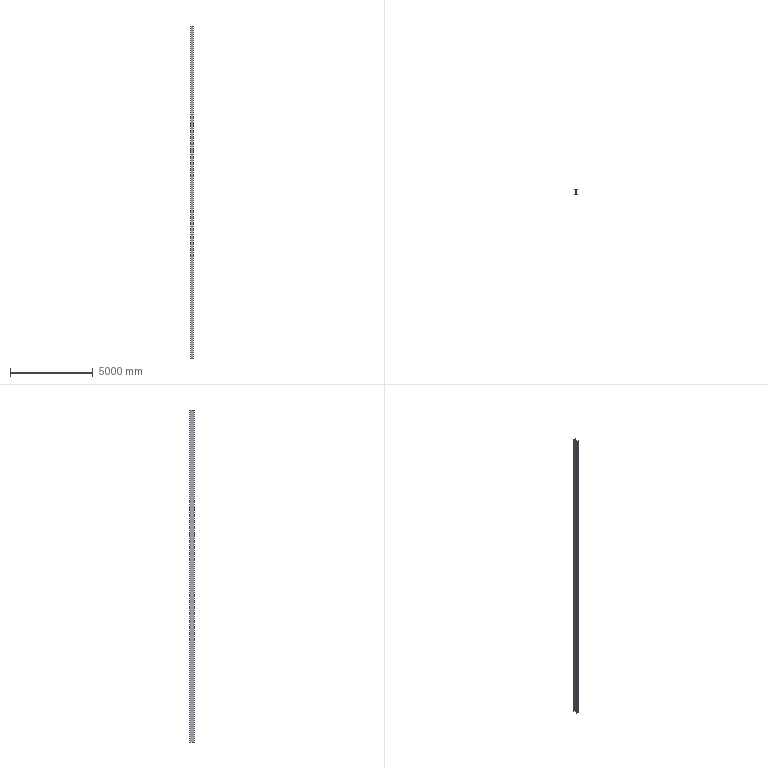Part | SolidWorks | features Extrusion 1 | 1 solid | 18 faces | box 150 x 300 x 20067 mm | volume 93874848 mm3 | plane 14 | cylinder 4 | commonest cylinder face diameters 26 x4
STEP:
#1=CARTESIAN_POINT('',(-75.,9.,0.));
#2=VERTEX_POINT('',#1);
#3=CARTESIAN_POINT('',(-75.,0.,0.));
#4=VERTEX_POINT('',#3);
#5=CARTESIAN_POINT('',(-75.,0.,0.));
#6=DIRECTION('',(0.,-1.,0.));
#7=VECTOR('',#6,1000.);
#8=LINE('',#5,#7);
#9=EDGE_CURVE('',#2,#4,#8,.T.);
#10=ORIENTED_EDGE('',*,*,#9,.T.);
#11=CARTESIAN_POINT('',(-75.,0.,20067.));
#12=VERTEX_POINT('',#11);
#13=CARTESIAN_POINT('',(-75.,0.,20067.));
#14=DIRECTION('',(0.,0.,-1.));
#15=VECTOR('',#14,1000.);
#16=LINE('',#13,#15);
#17=EDGE_CURVE('',#12,#4,#16,.T.);
#18=ORIENTED_EDGE('',*,*,#17,.F.);
#19=CARTESIAN_POINT('',(-75.,9.,20067.));
#20=VERTEX_POINT('',#19);
#21=CARTESIAN_POINT('',(-75.,0.,20067.));
#22=DIRECTION('',(0.,-1.,0.));
#23=VECTOR('',#22,1000.);
#24=LINE('',#21,#23);
#25=EDGE_CURVE('',#20,#12,#24,.T.);
#26=ORIENTED_EDGE('',*,*,#25,.F.);
#27=CARTESIAN_POINT('',(-75.,9.,20067.));
#28=DIRECTION('',(0.,0.,-1.));
#29=VECTOR('',#28,1000.);
#30=LINE('',#27,#29);
#31=EDGE_CURVE('',#20,#2,#30,.T.);
#32=ORIENTED_EDGE('',*,*,#31,.T.);
#33=EDGE_LOOP('',(#10,#18,#26,#32));
#34=FACE_OUTER_BOUND('',#33,.T.);
#35=CARTESIAN_POINT('',(-75.,0.,20067.));
#36=DIRECTION('',(1.,0.,0.));
#37=DIRECTION('',(0.,0.,-1.));
#38=AXIS2_PLACEMENT_3D('',#35,#36,#37);
#39=PLANE('',#38);
#40=ADVANCED_FACE('',(#34),#39,.F.);
#41=CARTESIAN_POINT('',(75.,0.,0.));
#42=VERTEX_POINT('',#41);
#43=CARTESIAN_POINT('',(75.,0.,0.));
#44=DIRECTION('',(1.,0.,0.));
#45=VECTOR('',#44,1000.);
#46=LINE('',#43,#45);
#47=EDGE_CURVE('',#4,#42,#46,.T.);
#48=ORIENTED_EDGE('',*,*,#47,.T.);
#49=CARTESIAN_POINT('',(75.,0.,20067.));
#50=VERTEX_POINT('',#49);
#51=CARTESIAN_POINT('',(75.,0.,20067.));
#52=DIRECTION('',(0.,0.,-1.));
#53=VECTOR('',#52,1000.);
#54=LINE('',#51,#53);
#55=EDGE_CURVE('',#50,#42,#54,.T.);
#56=ORIENTED_EDGE('',*,*,#55,.F.);
#57=CARTESIAN_POINT('',(75.,0.,20067.));
#58=DIRECTION('',(1.,0.,0.));
#59=VECTOR('',#58,1000.);
#60=LINE('',#57,#59);
#61=EDGE_CURVE('',#12,#50,#60,.T.);
#62=ORIENTED_EDGE('',*,*,#61,.F.);
#63=ORIENTED_EDGE('',*,*,#17,.T.);
#64=EDGE_LOOP('',(#48,#56,#62,#63));
#65=FACE_OUTER_BOUND('',#64,.T.);
#66=CARTESIAN_POINT('',(75.,0.,20067.));
#67=DIRECTION('',(0.,1.,0.));
#68=DIRECTION('',(-1.,0.,0.));
#69=AXIS2_PLACEMENT_3D('',#66,#67,#68);
#70=PLANE('',#69);
#71=ADVANCED_FACE('',(#65),#70,.F.);
#72=CARTESIAN_POINT('',(75.,9.,0.));
#73=VERTEX_POINT('',#72);
#74=CARTESIAN_POINT('',(75.,0.,0.));
#75=DIRECTION('',(0.,1.,0.));
#76=VECTOR('',#75,1000.);
#77=LINE('',#74,#76);
#78=EDGE_CURVE('',#42,#73,#77,.T.);
#79=ORIENTED_EDGE('',*,*,#78,.T.);
#80=CARTESIAN_POINT('',(75.,9.,20067.));
#81=VERTEX_POINT('',#80);
#82=CARTESIAN_POINT('',(75.,9.,20067.));
#83=DIRECTION('',(0.,0.,-1.));
#84=VECTOR('',#83,1000.);
#85=LINE('',#82,#84);
#86=EDGE_CURVE('',#81,#73,#85,.T.);
#87=ORIENTED_EDGE('',*,*,#86,.F.);
#88=CARTESIAN_POINT('',(75.,0.,20067.));
#89=DIRECTION('',(0.,1.,0.));
#90=VECTOR('',#89,1000.);
#91=LINE('',#88,#90);
#92=EDGE_CURVE('',#50,#81,#91,.T.);
#93=ORIENTED_EDGE('',*,*,#92,.F.);
#94=ORIENTED_EDGE('',*,*,#55,.T.);
#95=EDGE_LOOP('',(#79,#87,#93,#94));
#96=FACE_OUTER_BOUND('',#95,.T.);
#97=CARTESIAN_POINT('',(75.,0.,20067.));
#98=DIRECTION('',(-1.,0.,0.));
#99=DIRECTION('',(0.,0.,1.));
#100=AXIS2_PLACEMENT_3D('',#97,#98,#99);
#101=PLANE('',#100);
#102=ADVANCED_FACE('',(#96),#101,.F.);
#103=CARTESIAN_POINT('',(16.25,9.,0.));
#104=VERTEX_POINT('',#103);
#105=CARTESIAN_POINT('',(75.,9.,0.));
#106=DIRECTION('',(-1.,0.,0.));
#107=VECTOR('',#106,1000.);
#108=LINE('',#105,#107);
#109=EDGE_CURVE('',#73,#104,#108,.T.);
#110=ORIENTED_EDGE('',*,*,#109,.T.);
#111=CARTESIAN_POINT('',(16.25,9.,20067.));
#112=VERTEX_POINT('',#111);
#113=CARTESIAN_POINT('',(16.25,9.,20067.));
#114=DIRECTION('',(0.,0.,-1.));
#115=VECTOR('',#114,1000.);
#116=LINE('',#113,#115);
#117=EDGE_CURVE('',#112,#104,#116,.T.);
#118=ORIENTED_EDGE('',*,*,#117,.F.);
#119=CARTESIAN_POINT('',(75.,9.,20067.));
#120=DIRECTION('',(-1.,0.,0.));
#121=VECTOR('',#120,1000.);
#122=LINE('',#119,#121);
#123=EDGE_CURVE('',#81,#112,#122,.T.);
#124=ORIENTED_EDGE('',*,*,#123,.F.);
#125=ORIENTED_EDGE('',*,*,#86,.T.);
#126=EDGE_LOOP('',(#110,#118,#124,#125));
#127=FACE_OUTER_BOUND('',#126,.T.);
#128=CARTESIAN_POINT('',(75.,9.,20067.));
#129=DIRECTION('',(0.,-1.,0.));
#130=DIRECTION('',(1.,0.,0.));
#131=AXIS2_PLACEMENT_3D('',#128,#129,#130);
#132=PLANE('',#131);
#133=ADVANCED_FACE('',(#127),#132,.F.);
#134=CARTESIAN_POINT('',(3.25,22.,0.));
#135=VERTEX_POINT('',#134);
#136=CARTESIAN_POINT('',(16.25,22.,0.));
#137=DIRECTION('',(0.,0.,-1.));
#138=DIRECTION('',(-1.,0.,0.));
#139=AXIS2_PLACEMENT_3D('',#136,#137,#138);
#140=CIRCLE('',#139,13.);
#141=EDGE_CURVE('',#104,#135,#140,.T.);
#142=ORIENTED_EDGE('',*,*,#141,.T.);
#143=CARTESIAN_POINT('',(3.25,22.,20067.));
#144=VERTEX_POINT('',#143);
#145=CARTESIAN_POINT('',(3.25,22.,20067.));
#146=DIRECTION('',(0.,0.,-1.));
#147=VECTOR('',#146,1000.);
#148=LINE('',#145,#147);
#149=EDGE_CURVE('',#144,#135,#148,.T.);
#150=ORIENTED_EDGE('',*,*,#149,.F.);
#151=CARTESIAN_POINT('',(16.25,22.,20067.));
#152=DIRECTION('',(0.,0.,-1.));
#153=DIRECTION('',(-1.,0.,0.));
#154=AXIS2_PLACEMENT_3D('',#151,#152,#153);
#155=CIRCLE('',#154,13.);
#156=EDGE_CURVE('',#112,#144,#155,.T.);
#157=ORIENTED_EDGE('',*,*,#156,.F.);
#158=ORIENTED_EDGE('',*,*,#117,.T.);
#159=EDGE_LOOP('',(#142,#150,#157,#158));
#160=FACE_OUTER_BOUND('',#159,.T.);
#161=CARTESIAN_POINT('',(16.25,22.,20067.));
#162=DIRECTION('',(0.,0.,-1.));
#163=DIRECTION('',(-1.,0.,0.));
#164=AXIS2_PLACEMENT_3D('',#161,#162,#163);
#165=CYLINDRICAL_SURFACE('',#164,13.);
#166=ADVANCED_FACE('',(#160),#165,.F.);
#167=CARTESIAN_POINT('',(3.25,278.,0.));
#168=VERTEX_POINT('',#167);
#169=CARTESIAN_POINT('',(3.25,22.,0.));
#170=DIRECTION('',(0.,1.,0.));
#171=VECTOR('',#170,1000.);
#172=LINE('',#169,#171);
#173=EDGE_CURVE('',#135,#168,#172,.T.);
#174=ORIENTED_EDGE('',*,*,#173,.T.);
#175=CARTESIAN_POINT('',(3.25,278.,20067.));
#176=VERTEX_POINT('',#175);
#177=CARTESIAN_POINT('',(3.25,278.,20067.));
#178=DIRECTION('',(0.,0.,-1.));
#179=VECTOR('',#178,1000.);
#180=LINE('',#177,#179);
#181=EDGE_CURVE('',#176,#168,#180,.T.);
#182=ORIENTED_EDGE('',*,*,#181,.F.);
#183=CARTESIAN_POINT('',(3.25,22.,20067.));
#184=DIRECTION('',(0.,1.,0.));
#185=VECTOR('',#184,1000.);
#186=LINE('',#183,#185);
#187=EDGE_CURVE('',#144,#176,#186,.T.);
#188=ORIENTED_EDGE('',*,*,#187,.F.);
#189=ORIENTED_EDGE('',*,*,#149,.T.);
#190=EDGE_LOOP('',(#174,#182,#188,#189));
#191=FACE_OUTER_BOUND('',#190,.T.);
#192=CARTESIAN_POINT('',(3.25,22.,20067.));
#193=DIRECTION('',(-1.,0.,0.));
#194=DIRECTION('',(0.,0.,1.));
#195=AXIS2_PLACEMENT_3D('',#192,#193,#194);
#196=PLANE('',#195);
#197=ADVANCED_FACE('',(#191),#196,.F.);
#198=CARTESIAN_POINT('',(16.25,291.,0.));
#199=VERTEX_POINT('',#198);
#200=CARTESIAN_POINT('',(16.25,278.,0.));
#201=DIRECTION('',(0.,0.,-1.));
#202=DIRECTION('',(-1.,0.,0.));
#203=AXIS2_PLACEMENT_3D('',#200,#201,#202);
#204=CIRCLE('',#203,13.);
#205=EDGE_CURVE('',#168,#199,#204,.T.);
#206=ORIENTED_EDGE('',*,*,#205,.T.);
#207=CARTESIAN_POINT('',(16.25,291.,20067.));
#208=VERTEX_POINT('',#207);
#209=CARTESIAN_POINT('',(16.25,291.,20067.));
#210=DIRECTION('',(0.,0.,-1.));
#211=VECTOR('',#210,1000.);
#212=LINE('',#209,#211);
#213=EDGE_CURVE('',#208,#199,#212,.T.);
#214=ORIENTED_EDGE('',*,*,#213,.F.);
#215=CARTESIAN_POINT('',(16.25,278.,20067.));
#216=DIRECTION('',(0.,0.,-1.));
#217=DIRECTION('',(-1.,0.,0.));
#218=AXIS2_PLACEMENT_3D('',#215,#216,#217);
#219=CIRCLE('',#218,13.);
#220=EDGE_CURVE('',#176,#208,#219,.T.);
#221=ORIENTED_EDGE('',*,*,#220,.F.);
#222=ORIENTED_EDGE('',*,*,#181,.T.);
#223=EDGE_LOOP('',(#206,#214,#221,#222));
#224=FACE_OUTER_BOUND('',#223,.T.);
#225=CARTESIAN_POINT('',(16.25,278.,20067.));
#226=DIRECTION('',(0.,0.,-1.));
#227=DIRECTION('',(-1.,0.,0.));
#228=AXIS2_PLACEMENT_3D('',#225,#226,#227);
#229=CYLINDRICAL_SURFACE('',#228,13.);
#230=ADVANCED_FACE('',(#224),#229,.F.);
#231=CARTESIAN_POINT('',(75.,291.,0.));
#232=VERTEX_POINT('',#231);
#233=CARTESIAN_POINT('',(16.25,291.,0.));
#234=DIRECTION('',(1.,0.,0.));
#235=VECTOR('',#234,1000.);
#236=LINE('',#233,#235);
#237=EDGE_CURVE('',#199,#232,#236,.T.);
#238=ORIENTED_EDGE('',*,*,#237,.T.);
#239=CARTESIAN_POINT('',(75.,291.,20067.));
#240=VERTEX_POINT('',#239);
#241=CARTESIAN_POINT('',(75.,291.,20067.));
#242=DIRECTION('',(0.,0.,-1.));
#243=VECTOR('',#242,1000.);
#244=LINE('',#241,#243);
#245=EDGE_CURVE('',#240,#232,#244,.T.);
#246=ORIENTED_EDGE('',*,*,#245,.F.);
#247=CARTESIAN_POINT('',(16.25,291.,20067.));
#248=DIRECTION('',(1.,0.,0.));
#249=VECTOR('',#248,1000.);
#250=LINE('',#247,#249);
#251=EDGE_CURVE('',#208,#240,#250,.T.);
#252=ORIENTED_EDGE('',*,*,#251,.F.);
#253=ORIENTED_EDGE('',*,*,#213,.T.);
#254=EDGE_LOOP('',(#238,#246,#252,#253));
#255=FACE_OUTER_BOUND('',#254,.T.);
#256=CARTESIAN_POINT('',(16.25,291.,20067.));
#257=DIRECTION('',(0.,1.,0.));
#258=DIRECTION('',(-1.,0.,0.));
#259=AXIS2_PLACEMENT_3D('',#256,#257,#258);
#260=PLANE('',#259);
#261=ADVANCED_FACE('',(#255),#260,.F.);
#262=CARTESIAN_POINT('',(75.,300.,0.));
#263=VERTEX_POINT('',#262);
#264=CARTESIAN_POINT('',(75.,291.,0.));
#265=DIRECTION('',(0.,1.,0.));
#266=VECTOR('',#265,1000.);
#267=LINE('',#264,#266);
#268=EDGE_CURVE('',#232,#263,#267,.T.);
#269=ORIENTED_EDGE('',*,*,#268,.T.);
#270=CARTESIAN_POINT('',(75.,300.,20067.));
#271=VERTEX_POINT('',#270);
#272=CARTESIAN_POINT('',(75.,300.,20067.));
#273=DIRECTION('',(0.,0.,-1.));
#274=VECTOR('',#273,1000.);
#275=LINE('',#272,#274);
#276=EDGE_CURVE('',#271,#263,#275,.T.);
#277=ORIENTED_EDGE('',*,*,#276,.F.);
#278=CARTESIAN_POINT('',(75.,291.,20067.));
#279=DIRECTION('',(0.,1.,0.));
#280=VECTOR('',#279,1000.);
#281=LINE('',#278,#280);
#282=EDGE_CURVE('',#240,#271,#281,.T.);
#283=ORIENTED_EDGE('',*,*,#282,.F.);
#284=ORIENTED_EDGE('',*,*,#245,.T.);
#285=EDGE_LOOP('',(#269,#277,#283,#284));
#286=FACE_OUTER_BOUND('',#285,.T.);
#287=CARTESIAN_POINT('',(75.,291.,20067.));
#288=DIRECTION('',(-1.,0.,0.));
#289=DIRECTION('',(0.,-1.,0.));
#290=AXIS2_PLACEMENT_3D('',#287,#288,#289);
#291=PLANE('',#290);
#292=ADVANCED_FACE('',(#286),#291,.F.);
#293=CARTESIAN_POINT('',(-75.,300.,0.));
#294=VERTEX_POINT('',#293);
#295=CARTESIAN_POINT('',(-75.,300.,0.));
#296=DIRECTION('',(-1.,0.,0.));
#297=VECTOR('',#296,1000.);
#298=LINE('',#295,#297);
#299=EDGE_CURVE('',#263,#294,#298,.T.);
#300=ORIENTED_EDGE('',*,*,#299,.T.);
#301=CARTESIAN_POINT('',(-75.,300.,20067.));
#302=VERTEX_POINT('',#301);
#303=CARTESIAN_POINT('',(-75.,300.,20067.));
#304=DIRECTION('',(0.,0.,-1.));
#305=VECTOR('',#304,1000.);
#306=LINE('',#303,#305);
#307=EDGE_CURVE('',#302,#294,#306,.T.);
#308=ORIENTED_EDGE('',*,*,#307,.F.);
#309=CARTESIAN_POINT('',(-75.,300.,20067.));
#310=DIRECTION('',(-1.,0.,0.));
#311=VECTOR('',#310,1000.);
#312=LINE('',#309,#311);
#313=EDGE_CURVE('',#271,#302,#312,.T.);
#314=ORIENTED_EDGE('',*,*,#313,.F.);
#315=ORIENTED_EDGE('',*,*,#276,.T.);
#316=EDGE_LOOP('',(#300,#308,#314,#315));
#317=FACE_OUTER_BOUND('',#316,.T.);
#318=CARTESIAN_POINT('',(-75.,300.,20067.));
#319=DIRECTION('',(0.,-1.,0.));
#320=DIRECTION('',(0.,0.,-1.));
#321=AXIS2_PLACEMENT_3D('',#318,#319,#320);
#322=PLANE('',#321);
#323=ADVANCED_FACE('',(#317),#322,.F.);
#324=CARTESIAN_POINT('',(-75.,291.,0.));
#325=VERTEX_POINT('',#324);
#326=CARTESIAN_POINT('',(-75.,291.,0.));
#327=DIRECTION('',(0.,-1.,0.));
#328=VECTOR('',#327,1000.);
#329=LINE('',#326,#328);
#330=EDGE_CURVE('',#294,#325,#329,.T.);
#331=ORIENTED_EDGE('',*,*,#330,.T.);
#332=CARTESIAN_POINT('',(-75.,291.,20067.));
#333=VERTEX_POINT('',#332);
#334=CARTESIAN_POINT('',(-75.,291.,20067.));
#335=DIRECTION('',(0.,0.,-1.));
#336=VECTOR('',#335,1000.);
#337=LINE('',#334,#336);
#338=EDGE_CURVE('',#333,#325,#337,.T.);
#339=ORIENTED_EDGE('',*,*,#338,.F.);
#340=CARTESIAN_POINT('',(-75.,291.,20067.));
#341=DIRECTION('',(0.,-1.,0.));
#342=VECTOR('',#341,1000.);
#343=LINE('',#340,#342);
#344=EDGE_CURVE('',#302,#333,#343,.T.);
#345=ORIENTED_EDGE('',*,*,#344,.F.);
#346=ORIENTED_EDGE('',*,*,#307,.T.);
#347=EDGE_LOOP('',(#331,#339,#345,#346));
#348=FACE_OUTER_BOUND('',#347,.T.);
#349=CARTESIAN_POINT('',(-75.,291.,20067.));
#350=DIRECTION('',(1.,0.,0.));
#351=DIRECTION('',(0.,1.,0.));
#352=AXIS2_PLACEMENT_3D('',#349,#350,#351);
#353=PLANE('',#352);
#354=ADVANCED_FACE('',(#348),#353,.F.);
#355=CARTESIAN_POINT('',(-16.25,291.,0.));
#356=VERTEX_POINT('',#355);
#357=CARTESIAN_POINT('',(-16.25,291.,0.));
#358=DIRECTION('',(1.,0.,0.));
#359=VECTOR('',#358,1000.);
#360=LINE('',#357,#359);
#361=EDGE_CURVE('',#325,#356,#360,.T.);
#362=ORIENTED_EDGE('',*,*,#361,.T.);
#363=CARTESIAN_POINT('',(-16.25,291.,20067.));
#364=VERTEX_POINT('',#363);
#365=CARTESIAN_POINT('',(-16.25,291.,20067.));
#366=DIRECTION('',(0.,0.,-1.));
#367=VECTOR('',#366,1000.);
#368=LINE('',#365,#367);
#369=EDGE_CURVE('',#364,#356,#368,.T.);
#370=ORIENTED_EDGE('',*,*,#369,.F.);
#371=CARTESIAN_POINT('',(-16.25,291.,20067.));
#372=DIRECTION('',(1.,0.,0.));
#373=VECTOR('',#372,1000.);
#374=LINE('',#371,#373);
#375=EDGE_CURVE('',#333,#364,#374,.T.);
#376=ORIENTED_EDGE('',*,*,#375,.F.);
#377=ORIENTED_EDGE('',*,*,#338,.T.);
#378=EDGE_LOOP('',(#362,#370,#376,#377));
#379=FACE_OUTER_BOUND('',#378,.T.);
#380=CARTESIAN_POINT('',(-16.25,291.,20067.));
#381=DIRECTION('',(0.,1.,0.));
#382=DIRECTION('',(-1.,0.,0.));
#383=AXIS2_PLACEMENT_3D('',#380,#381,#382);
#384=PLANE('',#383);
#385=ADVANCED_FACE('',(#379),#384,.F.);
#386=CARTESIAN_POINT('',(-3.25,278.,0.));
#387=VERTEX_POINT('',#386);
#388=CARTESIAN_POINT('',(-16.25,278.,0.));
#389=DIRECTION('',(0.,0.,-1.));
#390=DIRECTION('',(1.,0.,0.));
#391=AXIS2_PLACEMENT_3D('',#388,#389,#390);
#392=CIRCLE('',#391,13.);
#393=EDGE_CURVE('',#356,#387,#392,.T.);
#394=ORIENTED_EDGE('',*,*,#393,.T.);
#395=CARTESIAN_POINT('',(-3.25,278.,20067.));
#396=VERTEX_POINT('',#395);
#397=CARTESIAN_POINT('',(-3.25,278.,20067.));
#398=DIRECTION('',(0.,0.,-1.));
#399=VECTOR('',#398,1000.);
#400=LINE('',#397,#399);
#401=EDGE_CURVE('',#396,#387,#400,.T.);
#402=ORIENTED_EDGE('',*,*,#401,.F.);
#403=CARTESIAN_POINT('',(-16.25,278.,20067.));
#404=DIRECTION('',(0.,0.,-1.));
#405=DIRECTION('',(1.,0.,0.));
#406=AXIS2_PLACEMENT_3D('',#403,#404,#405);
#407=CIRCLE('',#406,13.);
#408=EDGE_CURVE('',#364,#396,#407,.T.);
#409=ORIENTED_EDGE('',*,*,#408,.F.);
#410=ORIENTED_EDGE('',*,*,#369,.T.);
#411=EDGE_LOOP('',(#394,#402,#409,#410));
#412=FACE_OUTER_BOUND('',#411,.T.);
#413=CARTESIAN_POINT('',(-16.25,278.,20067.));
#414=DIRECTION('',(0.,0.,-1.));
#415=DIRECTION('',(-1.,0.,0.));
#416=AXIS2_PLACEMENT_3D('',#413,#414,#415);
#417=CYLINDRICAL_SURFACE('',#416,13.);
#418=ADVANCED_FACE('',(#412),#417,.F.);
#419=CARTESIAN_POINT('',(-3.25,22.,0.));
#420=VERTEX_POINT('',#419);
#421=CARTESIAN_POINT('',(-3.25,22.,0.));
#422=DIRECTION('',(0.,-1.,0.));
#423=VECTOR('',#422,1000.);
#424=LINE('',#421,#423);
#425=EDGE_CURVE('',#387,#420,#424,.T.);
#426=ORIENTED_EDGE('',*,*,#425,.T.);
#427=CARTESIAN_POINT('',(-3.25,22.,20067.));
#428=VERTEX_POINT('',#427);
#429=CARTESIAN_POINT('',(-3.25,22.,20067.));
#430=DIRECTION('',(0.,0.,-1.));
#431=VECTOR('',#430,1000.);
#432=LINE('',#429,#431);
#433=EDGE_CURVE('',#428,#420,#432,.T.);
#434=ORIENTED_EDGE('',*,*,#433,.F.);
#435=CARTESIAN_POINT('',(-3.25,22.,20067.));
#436=DIRECTION('',(0.,-1.,0.));
#437=VECTOR('',#436,1000.);
#438=LINE('',#435,#437);
#439=EDGE_CURVE('',#396,#428,#438,.T.);
#440=ORIENTED_EDGE('',*,*,#439,.F.);
#441=ORIENTED_EDGE('',*,*,#401,.T.);
#442=EDGE_LOOP('',(#426,#434,#440,#441));
#443=FACE_OUTER_BOUND('',#442,.T.);
#444=CARTESIAN_POINT('',(-3.25,22.,20067.));
#445=DIRECTION('',(1.,0.,0.));
#446=DIRECTION('',(0.,0.,-1.));
#447=AXIS2_PLACEMENT_3D('',#444,#445,#446);
#448=PLANE('',#447);
#449=ADVANCED_FACE('',(#443),#448,.F.);
#450=CARTESIAN_POINT('',(-16.25,9.,0.));
#451=VERTEX_POINT('',#450);
#452=CARTESIAN_POINT('',(-16.25,22.,0.));
#453=DIRECTION('',(0.,0.,-1.));
#454=DIRECTION('',(-1.,0.,0.));
#455=AXIS2_PLACEMENT_3D('',#452,#453,#454);
#456=CIRCLE('',#455,13.);
#457=EDGE_CURVE('',#420,#451,#456,.T.);
#458=ORIENTED_EDGE('',*,*,#457,.T.);
#459=CARTESIAN_POINT('',(-16.25,9.,20067.));
#460=VERTEX_POINT('',#459);
#461=CARTESIAN_POINT('',(-16.25,9.,20067.));
#462=DIRECTION('',(0.,0.,-1.));
#463=VECTOR('',#462,1000.);
#464=LINE('',#461,#463);
#465=EDGE_CURVE('',#460,#451,#464,.T.);
#466=ORIENTED_EDGE('',*,*,#465,.F.);
#467=CARTESIAN_POINT('',(-16.25,22.,20067.));
#468=DIRECTION('',(0.,0.,-1.));
#469=DIRECTION('',(-1.,0.,0.));
#470=AXIS2_PLACEMENT_3D('',#467,#468,#469);
#471=CIRCLE('',#470,13.);
#472=EDGE_CURVE('',#428,#460,#471,.T.);
#473=ORIENTED_EDGE('',*,*,#472,.F.);
#474=ORIENTED_EDGE('',*,*,#433,.T.);
#475=EDGE_LOOP('',(#458,#466,#473,#474));
#476=FACE_OUTER_BOUND('',#475,.T.);
#477=CARTESIAN_POINT('',(-16.25,22.,20067.));
#478=DIRECTION('',(0.,0.,-1.));
#479=DIRECTION('',(-1.,0.,0.));
#480=AXIS2_PLACEMENT_3D('',#477,#478,#479);
#481=CYLINDRICAL_SURFACE('',#480,13.);
#482=ADVANCED_FACE('',(#476),#481,.F.);
#483=CARTESIAN_POINT('',(-75.,9.,0.));
#484=DIRECTION('',(-1.,0.,0.));
#485=VECTOR('',#484,1000.);
#486=LINE('',#483,#485);
#487=EDGE_CURVE('',#451,#2,#486,.T.);
#488=ORIENTED_EDGE('',*,*,#487,.T.);
#489=ORIENTED_EDGE('',*,*,#31,.F.);
#490=CARTESIAN_POINT('',(-75.,9.,20067.));
#491=DIRECTION('',(-1.,0.,0.));
#492=VECTOR('',#491,1000.);
#493=LINE('',#490,#492);
#494=EDGE_CURVE('',#460,#20,#493,.T.);
#495=ORIENTED_EDGE('',*,*,#494,.F.);
#496=ORIENTED_EDGE('',*,*,#465,.T.);
#497=EDGE_LOOP('',(#488,#489,#495,#496));
#498=FACE_OUTER_BOUND('',#497,.T.);
#499=CARTESIAN_POINT('',(-75.,9.,20067.));
#500=DIRECTION('',(0.,-1.,0.));
#501=DIRECTION('',(1.,0.,0.));
#502=AXIS2_PLACEMENT_3D('',#499,#500,#501);
#503=PLANE('',#502);
#504=ADVANCED_FACE('',(#498),#503,.F.);
#505=ORIENTED_EDGE('',*,*,#25,.T.);
#506=ORIENTED_EDGE('',*,*,#61,.T.);
#507=ORIENTED_EDGE('',*,*,#92,.T.);
#508=ORIENTED_EDGE('',*,*,#123,.T.);
#509=ORIENTED_EDGE('',*,*,#156,.T.);
#510=ORIENTED_EDGE('',*,*,#187,.T.);
#511=ORIENTED_EDGE('',*,*,#220,.T.);
#512=ORIENTED_EDGE('',*,*,#251,.T.);
#513=ORIENTED_EDGE('',*,*,#282,.T.);
#514=ORIENTED_EDGE('',*,*,#313,.T.);
#515=ORIENTED_EDGE('',*,*,#344,.T.);
#516=ORIENTED_EDGE('',*,*,#375,.T.);
#517=ORIENTED_EDGE('',*,*,#408,.T.);
#518=ORIENTED_EDGE('',*,*,#439,.T.);
#519=ORIENTED_EDGE('',*,*,#472,.T.);
#520=ORIENTED_EDGE('',*,*,#494,.T.);
#521=EDGE_LOOP('',(#505,#506,#507,#508,#509,#510,#511,#512,#513,#514,#515,#516,#517,#518,#519,#520));
#522=FACE_OUTER_BOUND('',#521,.T.);
#523=CARTESIAN_POINT('',(-16.25,22.,20067.));
#524=DIRECTION('',(0.,0.,-1.));
#525=DIRECTION('',(-1.,0.,0.));
#526=AXIS2_PLACEMENT_3D('',#523,#524,#525);
#527=PLANE('',#526);
#528=ADVANCED_FACE('',(#522),#527,.F.);
#529=ORIENTED_EDGE('',*,*,#9,.F.);
#530=ORIENTED_EDGE('',*,*,#487,.F.);
#531=ORIENTED_EDGE('',*,*,#457,.F.);
#532=ORIENTED_EDGE('',*,*,#425,.F.);
#533=ORIENTED_EDGE('',*,*,#393,.F.);
#534=ORIENTED_EDGE('',*,*,#361,.F.);
#535=ORIENTED_EDGE('',*,*,#330,.F.);
#536=ORIENTED_EDGE('',*,*,#299,.F.);
#537=ORIENTED_EDGE('',*,*,#268,.F.);
#538=ORIENTED_EDGE('',*,*,#237,.F.);
#539=ORIENTED_EDGE('',*,*,#205,.F.);
#540=ORIENTED_EDGE('',*,*,#173,.F.);
#541=ORIENTED_EDGE('',*,*,#141,.F.);
#542=ORIENTED_EDGE('',*,*,#109,.F.);
#543=ORIENTED_EDGE('',*,*,#78,.F.);
#544=ORIENTED_EDGE('',*,*,#47,.F.);
#545=EDGE_LOOP('',(#529,#530,#531,#532,#533,#534,#535,#536,#537,#538,#539,#540,#541,#542,#543,#544));
#546=FACE_OUTER_BOUND('',#545,.T.);
#547=CARTESIAN_POINT('',(-16.25,22.,0.));
#548=DIRECTION('',(0.,0.,-1.));
#549=DIRECTION('',(-1.,0.,0.));
#550=AXIS2_PLACEMENT_3D('',#547,#548,#549);
#551=PLANE('',#550);
#552=ADVANCED_FACE('',(#546),#551,.T.);
#553=CLOSED_SHELL('',(#40,#71,#102,#133,#166,#197,#230,#261,#292,#323,#354,#385,#418,#449,#482,#504,#528,#552));
#554=MANIFOLD_SOLID_BREP('',#553);
#555=CARTESIAN_POINT('',(0.,0.,0.));
#556=DIRECTION('',(0.,0.,1.));
#557=DIRECTION('',(1.,0.,0.));
#558=AXIS2_PLACEMENT_3D('',#555,#556,#557);
#559=(LENGTH_UNIT()NAMED_UNIT(*)SI_UNIT(.MILLI.,.METRE.));
#560=UNCERTAINTY_MEASURE_WITH_UNIT(LENGTH_MEASURE(0.00001),#559,'','');
#561=(NAMED_UNIT(*)PLANE_ANGLE_UNIT()SI_UNIT($,.RADIAN.));
#562=(NAMED_UNIT(*)SI_UNIT($,.STERADIAN.)SOLID_ANGLE_UNIT());
#563=(GEOMETRIC_REPRESENTATION_CONTEXT(3)GLOBAL_UNCERTAINTY_ASSIGNED_CONTEXT((#560))GLOBAL_UNIT_ASSIGNED_CONTEXT((#559,#561,#562))REPRESENTATION_CONTEXT('',''));
#564=ADVANCED_BREP_SHAPE_REPRESENTATION('',(#554,#558),#563);